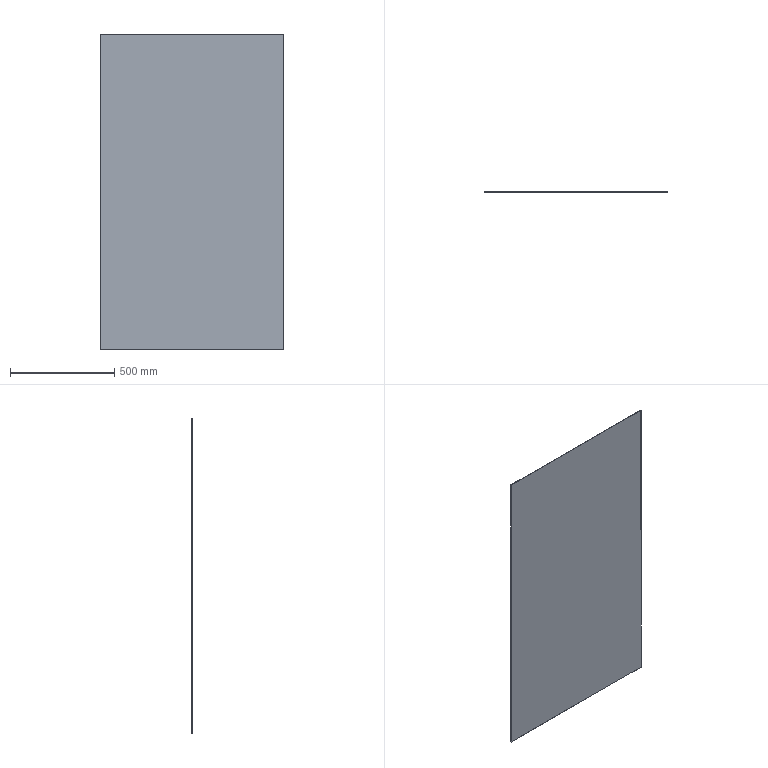Part | STEP file | PN_0020 Upper sealing plate | 1 solid | 6 faces | box 880 x 3 x 1510 mm | volume 3986400 mm3 | plane 6
STEP:
#1=CARTESIAN_POINT('',(0.,0.,0.));
#2=DIRECTION('',(0.,0.,1.));
#3=DIRECTION('',(1.,0.,0.));
#4=AXIS2_PLACEMENT_3D('',#1,#2,#3);
#5=CARTESIAN_POINT('',(0.,0.,0.));
#6=VERTEX_POINT('',#5);
#7=CARTESIAN_POINT('',(0.,0.,1510.));
#8=VERTEX_POINT('',#7);
#9=CARTESIAN_POINT('',(0.,0.,0.));
#10=DIRECTION('',(0.,0.,1.));
#11=VECTOR('',#10,1.);
#12=LINE('',#9,#11);
#13=CARTESIAN_POINT('',(0.,3.,0.));
#14=DIRECTION('',(1.,0.,0.));
#15=DIRECTION('',(0.,0.,-1.));
#16=AXIS2_PLACEMENT_3D('',#13,#14,#15);
#17=PLANE('',#16);
#18=CARTESIAN_POINT('',(0.,-3.));
#19=DIRECTION('',(-1.,0.));
#20=VECTOR('',#19,1.);
#21=LINE('',#18,#20);
#22=(GEOMETRIC_REPRESENTATION_CONTEXT(2)PARAMETRIC_REPRESENTATION_CONTEXT()REPRESENTATION_CONTEXT('',''));
#23=DEFINITIONAL_REPRESENTATION('',(#21),#22);
#24=PCURVE('',#17,#23);
#25=CARTESIAN_POINT('',(0.,0.,1510.));
#26=DIRECTION('',(0.,1.,0.));
#27=DIRECTION('',(0.,0.,1.));
#28=AXIS2_PLACEMENT_3D('',#25,#26,#27);
#29=PLANE('',#28);
#30=CARTESIAN_POINT('',(-1510.,0.));
#31=DIRECTION('',(1.,0.));
#32=VECTOR('',#31,1.);
#33=LINE('',#30,#32);
#34=(GEOMETRIC_REPRESENTATION_CONTEXT(2)PARAMETRIC_REPRESENTATION_CONTEXT()REPRESENTATION_CONTEXT('',''));
#35=DEFINITIONAL_REPRESENTATION('',(#33),#34);
#36=PCURVE('',#29,#35);
#37=SURFACE_CURVE('',#12,(#24,#36),.PCURVE_S1.);
#38=EDGE_CURVE('',#6,#8,#37,.T.);
#39=ORIENTED_EDGE('',*,*,#38,.T.);
#40=CARTESIAN_POINT('',(0.,3.,1510.));
#41=VERTEX_POINT('',#40);
#42=CARTESIAN_POINT('',(0.,3.,1510.));
#43=DIRECTION('',(0.,-1.,0.));
#44=VECTOR('',#43,1.);
#45=LINE('',#42,#44);
#46=CARTESIAN_POINT('',(-1510.,0.));
#47=DIRECTION('',(0.,-1.));
#48=VECTOR('',#47,1.);
#49=LINE('',#46,#48);
#50=(GEOMETRIC_REPRESENTATION_CONTEXT(2)PARAMETRIC_REPRESENTATION_CONTEXT()REPRESENTATION_CONTEXT('',''));
#51=DEFINITIONAL_REPRESENTATION('',(#49),#50);
#52=PCURVE('',#17,#51);
#53=CARTESIAN_POINT('',(0.,3.,1510.));
#54=DIRECTION('',(0.,0.,-1.));
#55=DIRECTION('',(-1.,0.,0.));
#56=AXIS2_PLACEMENT_3D('',#53,#54,#55);
#57=PLANE('',#56);
#58=CARTESIAN_POINT('',(0.,0.));
#59=DIRECTION('',(0.,-1.));
#60=VECTOR('',#59,1.);
#61=LINE('',#58,#60);
#62=(GEOMETRIC_REPRESENTATION_CONTEXT(2)PARAMETRIC_REPRESENTATION_CONTEXT()REPRESENTATION_CONTEXT('',''));
#63=DEFINITIONAL_REPRESENTATION('',(#61),#62);
#64=PCURVE('',#57,#63);
#65=SURFACE_CURVE('',#45,(#52,#64),.PCURVE_S1.);
#66=EDGE_CURVE('',#41,#8,#65,.T.);
#67=ORIENTED_EDGE('',*,*,#66,.F.);
#68=CARTESIAN_POINT('',(0.,3.,0.));
#69=VERTEX_POINT('',#68);
#70=CARTESIAN_POINT('',(0.,3.,0.));
#71=DIRECTION('',(0.,0.,1.));
#72=VECTOR('',#71,1.);
#73=LINE('',#70,#72);
#74=CARTESIAN_POINT('',(0.,0.));
#75=DIRECTION('',(-1.,0.));
#76=VECTOR('',#75,1.);
#77=LINE('',#74,#76);
#78=(GEOMETRIC_REPRESENTATION_CONTEXT(2)PARAMETRIC_REPRESENTATION_CONTEXT()REPRESENTATION_CONTEXT('',''));
#79=DEFINITIONAL_REPRESENTATION('',(#77),#78);
#80=PCURVE('',#17,#79);
#81=CARTESIAN_POINT('',(0.,3.,1510.));
#82=DIRECTION('',(0.,1.,0.));
#83=DIRECTION('',(0.,0.,1.));
#84=AXIS2_PLACEMENT_3D('',#81,#82,#83);
#85=PLANE('',#84);
#86=CARTESIAN_POINT('',(-1510.,0.));
#87=DIRECTION('',(1.,0.));
#88=VECTOR('',#87,1.);
#89=LINE('',#86,#88);
#90=(GEOMETRIC_REPRESENTATION_CONTEXT(2)PARAMETRIC_REPRESENTATION_CONTEXT()REPRESENTATION_CONTEXT('',''));
#91=DEFINITIONAL_REPRESENTATION('',(#89),#90);
#92=PCURVE('',#85,#91);
#93=SURFACE_CURVE('',#73,(#80,#92),.PCURVE_S1.);
#94=EDGE_CURVE('',#69,#41,#93,.T.);
#95=ORIENTED_EDGE('',*,*,#94,.F.);
#96=CARTESIAN_POINT('',(0.,3.,0.));
#97=DIRECTION('',(0.,-1.,0.));
#98=VECTOR('',#97,1.);
#99=LINE('',#96,#98);
#100=CARTESIAN_POINT('',(0.,0.));
#101=DIRECTION('',(0.,-1.));
#102=VECTOR('',#101,1.);
#103=LINE('',#100,#102);
#104=(GEOMETRIC_REPRESENTATION_CONTEXT(2)PARAMETRIC_REPRESENTATION_CONTEXT()REPRESENTATION_CONTEXT('',''));
#105=DEFINITIONAL_REPRESENTATION('',(#103),#104);
#106=PCURVE('',#17,#105);
#107=CARTESIAN_POINT('',(0.,3.,0.));
#108=DIRECTION('',(0.,0.,1.));
#109=DIRECTION('',(1.,0.,0.));
#110=AXIS2_PLACEMENT_3D('',#107,#108,#109);
#111=PLANE('',#110);
#112=CARTESIAN_POINT('',(0.,0.));
#113=DIRECTION('',(0.,-1.));
#114=VECTOR('',#113,1.);
#115=LINE('',#112,#114);
#116=(GEOMETRIC_REPRESENTATION_CONTEXT(2)PARAMETRIC_REPRESENTATION_CONTEXT()REPRESENTATION_CONTEXT('',''));
#117=DEFINITIONAL_REPRESENTATION('',(#115),#116);
#118=PCURVE('',#111,#117);
#119=SURFACE_CURVE('',#99,(#106,#118),.PCURVE_S1.);
#120=EDGE_CURVE('',#69,#6,#119,.T.);
#121=ORIENTED_EDGE('',*,*,#120,.T.);
#122=EDGE_LOOP('',(#39,#67,#95,#121));
#123=FACE_BOUND('',#122,.T.);
#124=ADVANCED_FACE('',(#123),#17,.F.);
#125=CARTESIAN_POINT('',(880.,0.,1510.));
#126=VERTEX_POINT('',#125);
#127=CARTESIAN_POINT('',(0.,0.,1510.));
#128=DIRECTION('',(1.,0.,0.));
#129=VECTOR('',#128,1.);
#130=LINE('',#127,#129);
#131=CARTESIAN_POINT('',(0.,-3.));
#132=DIRECTION('',(-1.,0.));
#133=VECTOR('',#132,1.);
#134=LINE('',#131,#133);
#135=(GEOMETRIC_REPRESENTATION_CONTEXT(2)PARAMETRIC_REPRESENTATION_CONTEXT()REPRESENTATION_CONTEXT('',''));
#136=DEFINITIONAL_REPRESENTATION('',(#134),#135);
#137=PCURVE('',#57,#136);
#138=CARTESIAN_POINT('',(0.,0.));
#139=DIRECTION('',(0.,1.));
#140=VECTOR('',#139,1.);
#141=LINE('',#138,#140);
#142=(GEOMETRIC_REPRESENTATION_CONTEXT(2)PARAMETRIC_REPRESENTATION_CONTEXT()REPRESENTATION_CONTEXT('',''));
#143=DEFINITIONAL_REPRESENTATION('',(#141),#142);
#144=PCURVE('',#29,#143);
#145=SURFACE_CURVE('',#130,(#137,#144),.PCURVE_S1.);
#146=EDGE_CURVE('',#8,#126,#145,.T.);
#147=ORIENTED_EDGE('',*,*,#146,.T.);
#148=CARTESIAN_POINT('',(880.,3.,1510.));
#149=VERTEX_POINT('',#148);
#150=CARTESIAN_POINT('',(880.,3.,1510.));
#151=DIRECTION('',(0.,-1.,0.));
#152=VECTOR('',#151,1.);
#153=LINE('',#150,#152);
#154=CARTESIAN_POINT('',(-880.,0.));
#155=DIRECTION('',(0.,-1.));
#156=VECTOR('',#155,1.);
#157=LINE('',#154,#156);
#158=(GEOMETRIC_REPRESENTATION_CONTEXT(2)PARAMETRIC_REPRESENTATION_CONTEXT()REPRESENTATION_CONTEXT('',''));
#159=DEFINITIONAL_REPRESENTATION('',(#157),#158);
#160=PCURVE('',#57,#159);
#161=CARTESIAN_POINT('',(880.,3.,0.));
#162=DIRECTION('',(-1.,0.,0.));
#163=DIRECTION('',(0.,0.,1.));
#164=AXIS2_PLACEMENT_3D('',#161,#162,#163);
#165=PLANE('',#164);
#166=CARTESIAN_POINT('',(1510.,0.));
#167=DIRECTION('',(0.,-1.));
#168=VECTOR('',#167,1.);
#169=LINE('',#166,#168);
#170=(GEOMETRIC_REPRESENTATION_CONTEXT(2)PARAMETRIC_REPRESENTATION_CONTEXT()REPRESENTATION_CONTEXT('',''));
#171=DEFINITIONAL_REPRESENTATION('',(#169),#170);
#172=PCURVE('',#165,#171);
#173=SURFACE_CURVE('',#153,(#160,#172),.PCURVE_S1.);
#174=EDGE_CURVE('',#149,#126,#173,.T.);
#175=ORIENTED_EDGE('',*,*,#174,.F.);
#176=CARTESIAN_POINT('',(0.,3.,1510.));
#177=DIRECTION('',(1.,0.,0.));
#178=VECTOR('',#177,1.);
#179=LINE('',#176,#178);
#180=CARTESIAN_POINT('',(0.,0.));
#181=DIRECTION('',(-1.,0.));
#182=VECTOR('',#181,1.);
#183=LINE('',#180,#182);
#184=(GEOMETRIC_REPRESENTATION_CONTEXT(2)PARAMETRIC_REPRESENTATION_CONTEXT()REPRESENTATION_CONTEXT('',''));
#185=DEFINITIONAL_REPRESENTATION('',(#183),#184);
#186=PCURVE('',#57,#185);
#187=CARTESIAN_POINT('',(0.,0.));
#188=DIRECTION('',(0.,1.));
#189=VECTOR('',#188,1.);
#190=LINE('',#187,#189);
#191=(GEOMETRIC_REPRESENTATION_CONTEXT(2)PARAMETRIC_REPRESENTATION_CONTEXT()REPRESENTATION_CONTEXT('',''));
#192=DEFINITIONAL_REPRESENTATION('',(#190),#191);
#193=PCURVE('',#85,#192);
#194=SURFACE_CURVE('',#179,(#186,#193),.PCURVE_S1.);
#195=EDGE_CURVE('',#41,#149,#194,.T.);
#196=ORIENTED_EDGE('',*,*,#195,.F.);
#197=ORIENTED_EDGE('',*,*,#66,.T.);
#198=EDGE_LOOP('',(#147,#175,#196,#197));
#199=FACE_BOUND('',#198,.T.);
#200=ADVANCED_FACE('',(#199),#57,.F.);
#201=CARTESIAN_POINT('',(880.,0.,0.));
#202=VERTEX_POINT('',#201);
#203=CARTESIAN_POINT('',(880.,0.,0.));
#204=DIRECTION('',(0.,0.,-1.));
#205=VECTOR('',#204,1.);
#206=LINE('',#203,#205);
#207=CARTESIAN_POINT('',(0.,-3.));
#208=DIRECTION('',(-1.,0.));
#209=VECTOR('',#208,1.);
#210=LINE('',#207,#209);
#211=(GEOMETRIC_REPRESENTATION_CONTEXT(2)PARAMETRIC_REPRESENTATION_CONTEXT()REPRESENTATION_CONTEXT('',''));
#212=DEFINITIONAL_REPRESENTATION('',(#210),#211);
#213=PCURVE('',#165,#212);
#214=CARTESIAN_POINT('',(-1510.,880.));
#215=DIRECTION('',(-1.,0.));
#216=VECTOR('',#215,1.);
#217=LINE('',#214,#216);
#218=(GEOMETRIC_REPRESENTATION_CONTEXT(2)PARAMETRIC_REPRESENTATION_CONTEXT()REPRESENTATION_CONTEXT('',''));
#219=DEFINITIONAL_REPRESENTATION('',(#217),#218);
#220=PCURVE('',#29,#219);
#221=SURFACE_CURVE('',#206,(#213,#220),.PCURVE_S1.);
#222=EDGE_CURVE('',#126,#202,#221,.T.);
#223=ORIENTED_EDGE('',*,*,#222,.T.);
#224=CARTESIAN_POINT('',(880.,3.,0.));
#225=VERTEX_POINT('',#224);
#226=CARTESIAN_POINT('',(880.,3.,0.));
#227=DIRECTION('',(0.,-1.,0.));
#228=VECTOR('',#227,1.);
#229=LINE('',#226,#228);
#230=CARTESIAN_POINT('',(0.,0.));
#231=DIRECTION('',(0.,-1.));
#232=VECTOR('',#231,1.);
#233=LINE('',#230,#232);
#234=(GEOMETRIC_REPRESENTATION_CONTEXT(2)PARAMETRIC_REPRESENTATION_CONTEXT()REPRESENTATION_CONTEXT('',''));
#235=DEFINITIONAL_REPRESENTATION('',(#233),#234);
#236=PCURVE('',#165,#235);
#237=CARTESIAN_POINT('',(880.,0.));
#238=DIRECTION('',(0.,-1.));
#239=VECTOR('',#238,1.);
#240=LINE('',#237,#239);
#241=(GEOMETRIC_REPRESENTATION_CONTEXT(2)PARAMETRIC_REPRESENTATION_CONTEXT()REPRESENTATION_CONTEXT('',''));
#242=DEFINITIONAL_REPRESENTATION('',(#240),#241);
#243=PCURVE('',#111,#242);
#244=SURFACE_CURVE('',#229,(#236,#243),.PCURVE_S1.);
#245=EDGE_CURVE('',#225,#202,#244,.T.);
#246=ORIENTED_EDGE('',*,*,#245,.F.);
#247=CARTESIAN_POINT('',(880.,3.,0.));
#248=DIRECTION('',(0.,0.,-1.));
#249=VECTOR('',#248,1.);
#250=LINE('',#247,#249);
#251=CARTESIAN_POINT('',(0.,0.));
#252=DIRECTION('',(-1.,0.));
#253=VECTOR('',#252,1.);
#254=LINE('',#251,#253);
#255=(GEOMETRIC_REPRESENTATION_CONTEXT(2)PARAMETRIC_REPRESENTATION_CONTEXT()REPRESENTATION_CONTEXT('',''));
#256=DEFINITIONAL_REPRESENTATION('',(#254),#255);
#257=PCURVE('',#165,#256);
#258=CARTESIAN_POINT('',(-1510.,880.));
#259=DIRECTION('',(-1.,0.));
#260=VECTOR('',#259,1.);
#261=LINE('',#258,#260);
#262=(GEOMETRIC_REPRESENTATION_CONTEXT(2)PARAMETRIC_REPRESENTATION_CONTEXT()REPRESENTATION_CONTEXT('',''));
#263=DEFINITIONAL_REPRESENTATION('',(#261),#262);
#264=PCURVE('',#85,#263);
#265=SURFACE_CURVE('',#250,(#257,#264),.PCURVE_S1.);
#266=EDGE_CURVE('',#149,#225,#265,.T.);
#267=ORIENTED_EDGE('',*,*,#266,.F.);
#268=ORIENTED_EDGE('',*,*,#174,.T.);
#269=EDGE_LOOP('',(#223,#246,#267,#268));
#270=FACE_BOUND('',#269,.T.);
#271=ADVANCED_FACE('',(#270),#165,.F.);
#272=CARTESIAN_POINT('',(0.,0.,0.));
#273=DIRECTION('',(-1.,0.,0.));
#274=VECTOR('',#273,1.);
#275=LINE('',#272,#274);
#276=CARTESIAN_POINT('',(0.,-3.));
#277=DIRECTION('',(-1.,0.));
#278=VECTOR('',#277,1.);
#279=LINE('',#276,#278);
#280=(GEOMETRIC_REPRESENTATION_CONTEXT(2)PARAMETRIC_REPRESENTATION_CONTEXT()REPRESENTATION_CONTEXT('',''));
#281=DEFINITIONAL_REPRESENTATION('',(#279),#280);
#282=PCURVE('',#111,#281);
#283=CARTESIAN_POINT('',(-1510.,0.));
#284=DIRECTION('',(0.,-1.));
#285=VECTOR('',#284,1.);
#286=LINE('',#283,#285);
#287=(GEOMETRIC_REPRESENTATION_CONTEXT(2)PARAMETRIC_REPRESENTATION_CONTEXT()REPRESENTATION_CONTEXT('',''));
#288=DEFINITIONAL_REPRESENTATION('',(#286),#287);
#289=PCURVE('',#29,#288);
#290=SURFACE_CURVE('',#275,(#282,#289),.PCURVE_S1.);
#291=EDGE_CURVE('',#202,#6,#290,.T.);
#292=ORIENTED_EDGE('',*,*,#291,.T.);
#293=ORIENTED_EDGE('',*,*,#120,.F.);
#294=CARTESIAN_POINT('',(0.,3.,0.));
#295=DIRECTION('',(-1.,0.,0.));
#296=VECTOR('',#295,1.);
#297=LINE('',#294,#296);
#298=CARTESIAN_POINT('',(0.,0.));
#299=DIRECTION('',(-1.,0.));
#300=VECTOR('',#299,1.);
#301=LINE('',#298,#300);
#302=(GEOMETRIC_REPRESENTATION_CONTEXT(2)PARAMETRIC_REPRESENTATION_CONTEXT()REPRESENTATION_CONTEXT('',''));
#303=DEFINITIONAL_REPRESENTATION('',(#301),#302);
#304=PCURVE('',#111,#303);
#305=CARTESIAN_POINT('',(-1510.,0.));
#306=DIRECTION('',(0.,-1.));
#307=VECTOR('',#306,1.);
#308=LINE('',#305,#307);
#309=(GEOMETRIC_REPRESENTATION_CONTEXT(2)PARAMETRIC_REPRESENTATION_CONTEXT()REPRESENTATION_CONTEXT('',''));
#310=DEFINITIONAL_REPRESENTATION('',(#308),#309);
#311=PCURVE('',#85,#310);
#312=SURFACE_CURVE('',#297,(#304,#311),.PCURVE_S1.);
#313=EDGE_CURVE('',#225,#69,#312,.T.);
#314=ORIENTED_EDGE('',*,*,#313,.F.);
#315=ORIENTED_EDGE('',*,*,#245,.T.);
#316=EDGE_LOOP('',(#292,#293,#314,#315));
#317=FACE_BOUND('',#316,.T.);
#318=ADVANCED_FACE('',(#317),#111,.F.);
#319=ORIENTED_EDGE('',*,*,#94,.T.);
#320=ORIENTED_EDGE('',*,*,#195,.T.);
#321=ORIENTED_EDGE('',*,*,#266,.T.);
#322=ORIENTED_EDGE('',*,*,#313,.T.);
#323=EDGE_LOOP('',(#319,#320,#321,#322));
#324=FACE_BOUND('',#323,.T.);
#325=ADVANCED_FACE('',(#324),#85,.T.);
#326=ORIENTED_EDGE('',*,*,#38,.F.);
#327=ORIENTED_EDGE('',*,*,#291,.F.);
#328=ORIENTED_EDGE('',*,*,#222,.F.);
#329=ORIENTED_EDGE('',*,*,#146,.F.);
#330=EDGE_LOOP('',(#326,#327,#328,#329));
#331=FACE_BOUND('',#330,.T.);
#332=ADVANCED_FACE('',(#331),#29,.F.);
#333=CLOSED_SHELL('',(#124,#200,#271,#318,#325,#332));
#334=MANIFOLD_SOLID_BREP('',#333);
#335=(LENGTH_UNIT()NAMED_UNIT(*)SI_UNIT(.MILLI.,.METRE.));
#336=UNCERTAINTY_MEASURE_WITH_UNIT(LENGTH_MEASURE(0.0000001),#335,'','');
#337=(NAMED_UNIT(*)PLANE_ANGLE_UNIT()SI_UNIT($,.RADIAN.));
#338=(NAMED_UNIT(*)SI_UNIT($,.STERADIAN.)SOLID_ANGLE_UNIT());
#339=(GEOMETRIC_REPRESENTATION_CONTEXT(3)GLOBAL_UNCERTAINTY_ASSIGNED_CONTEXT((#336))GLOBAL_UNIT_ASSIGNED_CONTEXT((#335,#337,#338))REPRESENTATION_CONTEXT('',''));
#340=ADVANCED_BREP_SHAPE_REPRESENTATION('',(#4,#334),#339);